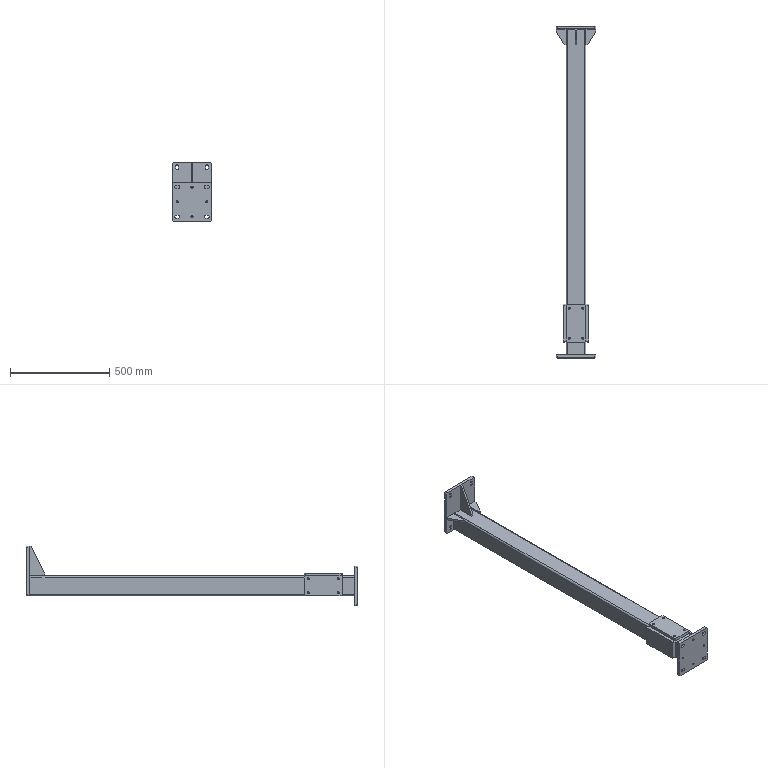Part | SolidWorks | features ICE 6, HoleWzd 4, CirPattern 2, DeleteBody 1, MirrorSolid 1, RefAxis 1, WeldCornerFeat 1, WeldMemberFeat 1, WeldmentFeature 1 | 9 solids | 165 faces | box 200 x 1668 x 300 mm | volume 4715517 mm3 | plane 97 | cylinder 68 | commonest cylinder face diameters 10.2 x40 13.5 x12 15 x8 8 x4 16 x4